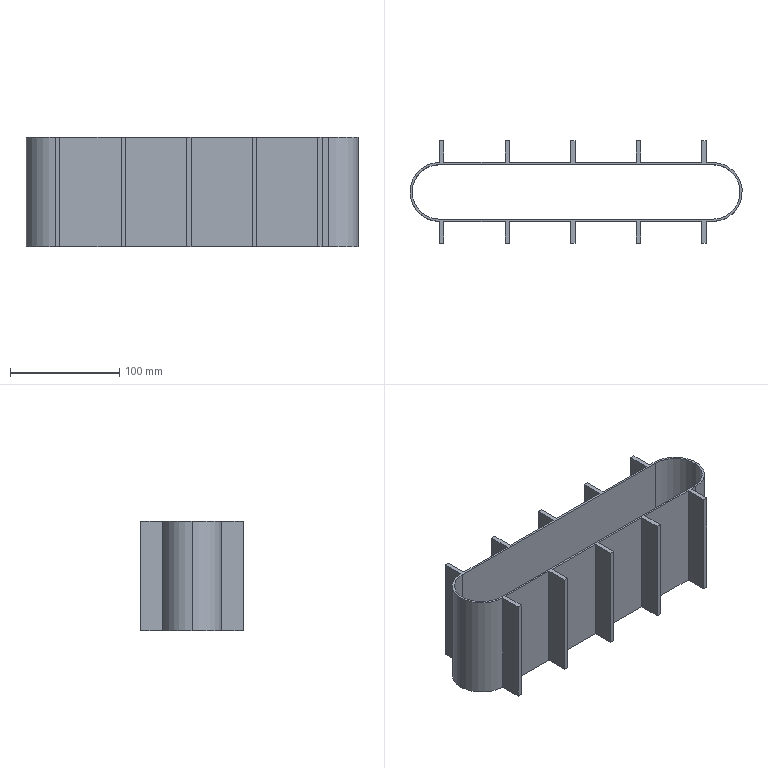Part | SolidWorks | features ICE 2, LPattern 2, Extrusion 1 | 1 solid | 50 faces | box 304 x 94 x 100 mm | volume 212673 mm3 | plane 44 | cylinder 6 | commonest cylinder face diameters 50 x3 54 x3
STEP:
#1=CARTESIAN_POINT('',(0.,25.,100.));
#2=VERTEX_POINT('',#1);
#3=CARTESIAN_POINT('',(-25.,0.,100.));
#4=VERTEX_POINT('',#3);
#5=CARTESIAN_POINT('',(0.,0.,100.));
#6=DIRECTION('',(0.,0.,1.));
#7=DIRECTION('',(1.,0.,0.));
#8=AXIS2_PLACEMENT_3D('',#5,#6,#7);
#9=CIRCLE('',#8,25.);
#10=EDGE_CURVE('',#2,#4,#9,.T.);
#11=ORIENTED_EDGE('',*,*,#10,.T.);
#12=CARTESIAN_POINT('',(-25.,0.,0.));
#13=VERTEX_POINT('',#12);
#14=CARTESIAN_POINT('',(-25.,0.,100.));
#15=DIRECTION('',(0.,0.,-1.));
#16=VECTOR('',#15,1000.);
#17=LINE('',#14,#16);
#18=EDGE_CURVE('',#4,#13,#17,.T.);
#19=ORIENTED_EDGE('',*,*,#18,.T.);
#20=CARTESIAN_POINT('',(0.,25.,0.));
#21=VERTEX_POINT('',#20);
#22=CARTESIAN_POINT('',(0.,0.,0.));
#23=DIRECTION('',(0.,0.,1.));
#24=DIRECTION('',(1.,0.,0.));
#25=AXIS2_PLACEMENT_3D('',#22,#23,#24);
#26=CIRCLE('',#25,25.);
#27=EDGE_CURVE('',#21,#13,#26,.T.);
#28=ORIENTED_EDGE('',*,*,#27,.F.);
#29=CARTESIAN_POINT('',(0.,25.,100.));
#30=DIRECTION('',(0.,0.,-1.));
#31=VECTOR('',#30,1000.);
#32=LINE('',#29,#31);
#33=EDGE_CURVE('',#2,#21,#32,.T.);
#34=ORIENTED_EDGE('',*,*,#33,.F.);
#35=EDGE_LOOP('',(#11,#19,#28,#34));
#36=FACE_OUTER_BOUND('',#35,.T.);
#37=CARTESIAN_POINT('',(0.,0.,100.));
#38=DIRECTION('',(0.,0.,-1.));
#39=DIRECTION('',(-1.,0.,0.));
#40=AXIS2_PLACEMENT_3D('',#37,#38,#39);
#41=CYLINDRICAL_SURFACE('',#40,25.);
#42=ADVANCED_FACE('',(#36),#41,.F.);
#43=CARTESIAN_POINT('',(-27.,0.,100.));
#44=VERTEX_POINT('',#43);
#45=CARTESIAN_POINT('',(0.,-27.,100.));
#46=VERTEX_POINT('',#45);
#47=CARTESIAN_POINT('',(0.,0.,100.));
#48=DIRECTION('',(0.,0.,1.));
#49=DIRECTION('',(1.,0.,0.));
#50=AXIS2_PLACEMENT_3D('',#47,#48,#49);
#51=CIRCLE('',#50,27.);
#52=EDGE_CURVE('',#44,#46,#51,.T.);
#53=ORIENTED_EDGE('',*,*,#52,.F.);
#54=CARTESIAN_POINT('',(-27.,0.,0.));
#55=VERTEX_POINT('',#54);
#56=CARTESIAN_POINT('',(-27.,0.,100.));
#57=DIRECTION('',(0.,0.,-1.));
#58=VECTOR('',#57,1000.);
#59=LINE('',#56,#58);
#60=EDGE_CURVE('',#44,#55,#59,.T.);
#61=ORIENTED_EDGE('',*,*,#60,.T.);
#62=CARTESIAN_POINT('',(0.,-27.,0.));
#63=VERTEX_POINT('',#62);
#64=CARTESIAN_POINT('',(0.,0.,0.));
#65=DIRECTION('',(0.,0.,1.));
#66=DIRECTION('',(1.,0.,0.));
#67=AXIS2_PLACEMENT_3D('',#64,#65,#66);
#68=CIRCLE('',#67,27.);
#69=EDGE_CURVE('',#55,#63,#68,.T.);
#70=ORIENTED_EDGE('',*,*,#69,.T.);
#71=CARTESIAN_POINT('',(0.,-27.,100.));
#72=DIRECTION('',(0.,0.,-1.));
#73=VECTOR('',#72,1000.);
#74=LINE('',#71,#73);
#75=EDGE_CURVE('',#46,#63,#74,.T.);
#76=ORIENTED_EDGE('',*,*,#75,.F.);
#77=EDGE_LOOP('',(#53,#61,#70,#76));
#78=FACE_OUTER_BOUND('',#77,.T.);
#79=CARTESIAN_POINT('',(0.,0.,100.));
#80=DIRECTION('',(0.,0.,-1.));
#81=DIRECTION('',(-1.,0.,0.));
#82=AXIS2_PLACEMENT_3D('',#79,#80,#81);
#83=CYLINDRICAL_SURFACE('',#82,27.);
#84=ADVANCED_FACE('',(#78),#83,.T.);
#85=CARTESIAN_POINT('',(184.,-27.,0.));
#86=VERTEX_POINT('',#85);
#87=CARTESIAN_POINT('',(240.,-27.,0.));
#88=VERTEX_POINT('',#87);
#89=CARTESIAN_POINT('',(0.,-27.,0.));
#90=DIRECTION('',(1.,0.,0.));
#91=VECTOR('',#90,1000.);
#92=LINE('',#89,#91);
#93=EDGE_CURVE('',#86,#88,#92,.T.);
#94=ORIENTED_EDGE('',*,*,#93,.T.);
#95=CARTESIAN_POINT('',(240.,-27.,100.));
#96=VERTEX_POINT('',#95);
#97=CARTESIAN_POINT('',(240.,-27.,-20.396));
#98=DIRECTION('',(0.,0.,1.));
#99=VECTOR('',#98,1000.);
#100=LINE('',#97,#99);
#101=EDGE_CURVE('',#88,#96,#100,.T.);
#102=ORIENTED_EDGE('',*,*,#101,.T.);
#103=CARTESIAN_POINT('',(184.,-27.,100.));
#104=VERTEX_POINT('',#103);
#105=CARTESIAN_POINT('',(0.,-27.,100.));
#106=DIRECTION('',(1.,0.,0.));
#107=VECTOR('',#106,1000.);
#108=LINE('',#105,#107);
#109=EDGE_CURVE('',#104,#96,#108,.T.);
#110=ORIENTED_EDGE('',*,*,#109,.F.);
#111=CARTESIAN_POINT('',(184.,-27.,-20.396));
#112=DIRECTION('',(0.,0.,1.));
#113=VECTOR('',#112,1000.);
#114=LINE('',#111,#113);
#115=EDGE_CURVE('',#86,#104,#114,.T.);
#116=ORIENTED_EDGE('',*,*,#115,.F.);
#117=EDGE_LOOP('',(#94,#102,#110,#116));
#118=FACE_OUTER_BOUND('',#117,.T.);
#119=CARTESIAN_POINT('',(0.,-27.,100.));
#120=DIRECTION('',(0.,1.,0.));
#121=DIRECTION('',(0.,0.,1.));
#122=AXIS2_PLACEMENT_3D('',#119,#120,#121);
#123=PLANE('',#122);
#124=ADVANCED_FACE('',(#118),#123,.F.);
#125=CARTESIAN_POINT('',(124.,-27.,0.));
#126=VERTEX_POINT('',#125);
#127=CARTESIAN_POINT('',(180.,-27.,0.));
#128=VERTEX_POINT('',#127);
#129=CARTESIAN_POINT('',(0.,-27.,0.));
#130=DIRECTION('',(1.,0.,0.));
#131=VECTOR('',#130,1000.);
#132=LINE('',#129,#131);
#133=EDGE_CURVE('',#126,#128,#132,.T.);
#134=ORIENTED_EDGE('',*,*,#133,.T.);
#135=CARTESIAN_POINT('',(180.,-27.,100.));
#136=VERTEX_POINT('',#135);
#137=CARTESIAN_POINT('',(180.,-27.,-20.396));
#138=DIRECTION('',(0.,0.,1.));
#139=VECTOR('',#138,1000.);
#140=LINE('',#137,#139);
#141=EDGE_CURVE('',#128,#136,#140,.T.);
#142=ORIENTED_EDGE('',*,*,#141,.T.);
#143=CARTESIAN_POINT('',(124.,-27.,100.));
#144=VERTEX_POINT('',#143);
#145=CARTESIAN_POINT('',(0.,-27.,100.));
#146=DIRECTION('',(1.,0.,0.));
#147=VECTOR('',#146,1000.);
#148=LINE('',#145,#147);
#149=EDGE_CURVE('',#144,#136,#148,.T.);
#150=ORIENTED_EDGE('',*,*,#149,.F.);
#151=CARTESIAN_POINT('',(124.,-27.,-20.396));
#152=DIRECTION('',(0.,0.,1.));
#153=VECTOR('',#152,1000.);
#154=LINE('',#151,#153);
#155=EDGE_CURVE('',#126,#144,#154,.T.);
#156=ORIENTED_EDGE('',*,*,#155,.F.);
#157=EDGE_LOOP('',(#134,#142,#150,#156));
#158=FACE_OUTER_BOUND('',#157,.T.);
#159=CARTESIAN_POINT('',(0.,-27.,100.));
#160=DIRECTION('',(0.,1.,0.));
#161=DIRECTION('',(0.,0.,1.));
#162=AXIS2_PLACEMENT_3D('',#159,#160,#161);
#163=PLANE('',#162);
#164=ADVANCED_FACE('',(#158),#163,.F.);
#165=CARTESIAN_POINT('',(64.,-27.,0.));
#166=VERTEX_POINT('',#165);
#167=CARTESIAN_POINT('',(120.,-27.,0.));
#168=VERTEX_POINT('',#167);
#169=CARTESIAN_POINT('',(0.,-27.,0.));
#170=DIRECTION('',(1.,0.,0.));
#171=VECTOR('',#170,1000.);
#172=LINE('',#169,#171);
#173=EDGE_CURVE('',#166,#168,#172,.T.);
#174=ORIENTED_EDGE('',*,*,#173,.T.);
#175=CARTESIAN_POINT('',(120.,-27.,100.));
#176=VERTEX_POINT('',#175);
#177=CARTESIAN_POINT('',(120.,-27.,-20.396));
#178=DIRECTION('',(0.,0.,1.));
#179=VECTOR('',#178,1000.);
#180=LINE('',#177,#179);
#181=EDGE_CURVE('',#168,#176,#180,.T.);
#182=ORIENTED_EDGE('',*,*,#181,.T.);
#183=CARTESIAN_POINT('',(64.,-27.,100.));
#184=VERTEX_POINT('',#183);
#185=CARTESIAN_POINT('',(0.,-27.,100.));
#186=DIRECTION('',(1.,0.,0.));
#187=VECTOR('',#186,1000.);
#188=LINE('',#185,#187);
#189=EDGE_CURVE('',#184,#176,#188,.T.);
#190=ORIENTED_EDGE('',*,*,#189,.F.);
#191=CARTESIAN_POINT('',(64.,-27.,-20.396));
#192=DIRECTION('',(0.,0.,1.));
#193=VECTOR('',#192,1000.);
#194=LINE('',#191,#193);
#195=EDGE_CURVE('',#166,#184,#194,.T.);
#196=ORIENTED_EDGE('',*,*,#195,.F.);
#197=EDGE_LOOP('',(#174,#182,#190,#196));
#198=FACE_OUTER_BOUND('',#197,.T.);
#199=CARTESIAN_POINT('',(0.,-27.,100.));
#200=DIRECTION('',(0.,1.,0.));
#201=DIRECTION('',(0.,0.,1.));
#202=AXIS2_PLACEMENT_3D('',#199,#200,#201);
#203=PLANE('',#202);
#204=ADVANCED_FACE('',(#198),#203,.F.);
#205=CARTESIAN_POINT('',(4.,-27.,0.));
#206=VERTEX_POINT('',#205);
#207=CARTESIAN_POINT('',(60.,-27.,0.));
#208=VERTEX_POINT('',#207);
#209=CARTESIAN_POINT('',(0.,-27.,0.));
#210=DIRECTION('',(1.,0.,0.));
#211=VECTOR('',#210,1000.);
#212=LINE('',#209,#211);
#213=EDGE_CURVE('',#206,#208,#212,.T.);
#214=ORIENTED_EDGE('',*,*,#213,.T.);
#215=CARTESIAN_POINT('',(60.,-27.,100.));
#216=VERTEX_POINT('',#215);
#217=CARTESIAN_POINT('',(60.,-27.,-20.396));
#218=DIRECTION('',(0.,0.,1.));
#219=VECTOR('',#218,1000.);
#220=LINE('',#217,#219);
#221=EDGE_CURVE('',#208,#216,#220,.T.);
#222=ORIENTED_EDGE('',*,*,#221,.T.);
#223=CARTESIAN_POINT('',(4.,-27.,100.));
#224=VERTEX_POINT('',#223);
#225=CARTESIAN_POINT('',(0.,-27.,100.));
#226=DIRECTION('',(1.,0.,0.));
#227=VECTOR('',#226,1000.);
#228=LINE('',#225,#227);
#229=EDGE_CURVE('',#224,#216,#228,.T.);
#230=ORIENTED_EDGE('',*,*,#229,.F.);
#231=CARTESIAN_POINT('',(4.,-27.,-20.396));
#232=DIRECTION('',(0.,0.,1.));
#233=VECTOR('',#232,1000.);
#234=LINE('',#231,#233);
#235=EDGE_CURVE('',#206,#224,#234,.T.);
#236=ORIENTED_EDGE('',*,*,#235,.F.);
#237=EDGE_LOOP('',(#214,#222,#230,#236));
#238=FACE_OUTER_BOUND('',#237,.T.);
#239=CARTESIAN_POINT('',(0.,-27.,100.));
#240=DIRECTION('',(0.,1.,0.));
#241=DIRECTION('',(0.,0.,1.));
#242=AXIS2_PLACEMENT_3D('',#239,#240,#241);
#243=PLANE('',#242);
#244=ADVANCED_FACE('',(#238),#243,.F.);
#245=CARTESIAN_POINT('',(240.,27.,100.));
#246=VERTEX_POINT('',#245);
#247=CARTESIAN_POINT('',(184.,27.,100.));
#248=VERTEX_POINT('',#247);
#249=CARTESIAN_POINT('',(0.,27.,100.));
#250=DIRECTION('',(-1.,0.,0.));
#251=VECTOR('',#250,1000.);
#252=LINE('',#249,#251);
#253=EDGE_CURVE('',#246,#248,#252,.T.);
#254=ORIENTED_EDGE('',*,*,#253,.F.);
#255=CARTESIAN_POINT('',(240.,27.,0.));
#256=VERTEX_POINT('',#255);
#257=CARTESIAN_POINT('',(240.,27.,-20.396));
#258=DIRECTION('',(0.,0.,1.));
#259=VECTOR('',#258,1000.);
#260=LINE('',#257,#259);
#261=EDGE_CURVE('',#256,#246,#260,.T.);
#262=ORIENTED_EDGE('',*,*,#261,.F.);
#263=CARTESIAN_POINT('',(184.,27.,0.));
#264=VERTEX_POINT('',#263);
#265=CARTESIAN_POINT('',(0.,27.,0.));
#266=DIRECTION('',(-1.,0.,0.));
#267=VECTOR('',#266,1000.);
#268=LINE('',#265,#267);
#269=EDGE_CURVE('',#256,#264,#268,.T.);
#270=ORIENTED_EDGE('',*,*,#269,.T.);
#271=CARTESIAN_POINT('',(184.,27.,-20.396));
#272=DIRECTION('',(0.,0.,1.));
#273=VECTOR('',#272,1000.);
#274=LINE('',#271,#273);
#275=EDGE_CURVE('',#264,#248,#274,.T.);
#276=ORIENTED_EDGE('',*,*,#275,.T.);
#277=EDGE_LOOP('',(#254,#262,#270,#276));
#278=FACE_OUTER_BOUND('',#277,.T.);
#279=CARTESIAN_POINT('',(0.,27.,100.));
#280=DIRECTION('',(0.,-1.,0.));
#281=DIRECTION('',(0.,0.,-1.));
#282=AXIS2_PLACEMENT_3D('',#279,#280,#281);
#283=PLANE('',#282);
#284=ADVANCED_FACE('',(#278),#283,.F.);
#285=CARTESIAN_POINT('',(180.,27.,100.));
#286=VERTEX_POINT('',#285);
#287=CARTESIAN_POINT('',(124.,27.,100.));
#288=VERTEX_POINT('',#287);
#289=CARTESIAN_POINT('',(0.,27.,100.));
#290=DIRECTION('',(-1.,0.,0.));
#291=VECTOR('',#290,1000.);
#292=LINE('',#289,#291);
#293=EDGE_CURVE('',#286,#288,#292,.T.);
#294=ORIENTED_EDGE('',*,*,#293,.F.);
#295=CARTESIAN_POINT('',(180.,27.,0.));
#296=VERTEX_POINT('',#295);
#297=CARTESIAN_POINT('',(180.,27.,-20.396));
#298=DIRECTION('',(0.,0.,1.));
#299=VECTOR('',#298,1000.);
#300=LINE('',#297,#299);
#301=EDGE_CURVE('',#296,#286,#300,.T.);
#302=ORIENTED_EDGE('',*,*,#301,.F.);
#303=CARTESIAN_POINT('',(124.,27.,0.));
#304=VERTEX_POINT('',#303);
#305=CARTESIAN_POINT('',(0.,27.,0.));
#306=DIRECTION('',(-1.,0.,0.));
#307=VECTOR('',#306,1000.);
#308=LINE('',#305,#307);
#309=EDGE_CURVE('',#296,#304,#308,.T.);
#310=ORIENTED_EDGE('',*,*,#309,.T.);
#311=CARTESIAN_POINT('',(124.,27.,-20.396));
#312=DIRECTION('',(0.,0.,1.));
#313=VECTOR('',#312,1000.);
#314=LINE('',#311,#313);
#315=EDGE_CURVE('',#304,#288,#314,.T.);
#316=ORIENTED_EDGE('',*,*,#315,.T.);
#317=EDGE_LOOP('',(#294,#302,#310,#316));
#318=FACE_OUTER_BOUND('',#317,.T.);
#319=CARTESIAN_POINT('',(0.,27.,100.));
#320=DIRECTION('',(0.,-1.,0.));
#321=DIRECTION('',(0.,0.,-1.));
#322=AXIS2_PLACEMENT_3D('',#319,#320,#321);
#323=PLANE('',#322);
#324=ADVANCED_FACE('',(#318),#323,.F.);
#325=CARTESIAN_POINT('',(120.,27.,100.));
#326=VERTEX_POINT('',#325);
#327=CARTESIAN_POINT('',(64.,27.,100.));
#328=VERTEX_POINT('',#327);
#329=CARTESIAN_POINT('',(0.,27.,100.));
#330=DIRECTION('',(-1.,0.,0.));
#331=VECTOR('',#330,1000.);
#332=LINE('',#329,#331);
#333=EDGE_CURVE('',#326,#328,#332,.T.);
#334=ORIENTED_EDGE('',*,*,#333,.F.);
#335=CARTESIAN_POINT('',(120.,27.,0.));
#336=VERTEX_POINT('',#335);
#337=CARTESIAN_POINT('',(120.,27.,-20.396));
#338=DIRECTION('',(0.,0.,1.));
#339=VECTOR('',#338,1000.);
#340=LINE('',#337,#339);
#341=EDGE_CURVE('',#336,#326,#340,.T.);
#342=ORIENTED_EDGE('',*,*,#341,.F.);
#343=CARTESIAN_POINT('',(64.,27.,0.));
#344=VERTEX_POINT('',#343);
#345=CARTESIAN_POINT('',(0.,27.,0.));
#346=DIRECTION('',(-1.,0.,0.));
#347=VECTOR('',#346,1000.);
#348=LINE('',#345,#347);
#349=EDGE_CURVE('',#336,#344,#348,.T.);
#350=ORIENTED_EDGE('',*,*,#349,.T.);
#351=CARTESIAN_POINT('',(64.,27.,-20.396));
#352=DIRECTION('',(0.,0.,1.));
#353=VECTOR('',#352,1000.);
#354=LINE('',#351,#353);
#355=EDGE_CURVE('',#344,#328,#354,.T.);
#356=ORIENTED_EDGE('',*,*,#355,.T.);
#357=EDGE_LOOP('',(#334,#342,#350,#356));
#358=FACE_OUTER_BOUND('',#357,.T.);
#359=CARTESIAN_POINT('',(0.,27.,100.));
#360=DIRECTION('',(0.,-1.,0.));
#361=DIRECTION('',(0.,0.,-1.));
#362=AXIS2_PLACEMENT_3D('',#359,#360,#361);
#363=PLANE('',#362);
#364=ADVANCED_FACE('',(#358),#363,.F.);
#365=CARTESIAN_POINT('',(60.,27.,100.));
#366=VERTEX_POINT('',#365);
#367=CARTESIAN_POINT('',(4.,27.,100.));
#368=VERTEX_POINT('',#367);
#369=CARTESIAN_POINT('',(0.,27.,100.));
#370=DIRECTION('',(-1.,0.,0.));
#371=VECTOR('',#370,1000.);
#372=LINE('',#369,#371);
#373=EDGE_CURVE('',#366,#368,#372,.T.);
#374=ORIENTED_EDGE('',*,*,#373,.F.);
#375=CARTESIAN_POINT('',(60.,27.,0.));
#376=VERTEX_POINT('',#375);
#377=CARTESIAN_POINT('',(60.,27.,-20.396));
#378=DIRECTION('',(0.,0.,1.));
#379=VECTOR('',#378,1000.);
#380=LINE('',#377,#379);
#381=EDGE_CURVE('',#376,#366,#380,.T.);
#382=ORIENTED_EDGE('',*,*,#381,.F.);
#383=CARTESIAN_POINT('',(4.,27.,0.));
#384=VERTEX_POINT('',#383);
#385=CARTESIAN_POINT('',(0.,27.,0.));
#386=DIRECTION('',(-1.,0.,0.));
#387=VECTOR('',#386,1000.);
#388=LINE('',#385,#387);
#389=EDGE_CURVE('',#376,#384,#388,.T.);
#390=ORIENTED_EDGE('',*,*,#389,.T.);
#391=CARTESIAN_POINT('',(4.,27.,-20.396));
#392=DIRECTION('',(0.,0.,1.));
#393=VECTOR('',#392,1000.);
#394=LINE('',#391,#393);
#395=EDGE_CURVE('',#384,#368,#394,.T.);
#396=ORIENTED_EDGE('',*,*,#395,.T.);
#397=EDGE_LOOP('',(#374,#382,#390,#396));
#398=FACE_OUTER_BOUND('',#397,.T.);
#399=CARTESIAN_POINT('',(0.,27.,100.));
#400=DIRECTION('',(0.,-1.,0.));
#401=DIRECTION('',(0.,0.,-1.));
#402=AXIS2_PLACEMENT_3D('',#399,#400,#401);
#403=PLANE('',#402);
#404=ADVANCED_FACE('',(#398),#403,.F.);
#405=CARTESIAN_POINT('',(0.,27.,100.));
#406=VERTEX_POINT('',#405);
#407=CARTESIAN_POINT('',(0.,0.,100.));
#408=DIRECTION('',(0.,0.,1.));
#409=DIRECTION('',(1.,0.,0.));
#410=AXIS2_PLACEMENT_3D('',#407,#408,#409);
#411=CIRCLE('',#410,27.);
#412=EDGE_CURVE('',#406,#44,#411,.T.);
#413=ORIENTED_EDGE('',*,*,#412,.T.);
#414=ORIENTED_EDGE('',*,*,#52,.T.);
#415=CARTESIAN_POINT('',(0.,-47.,100.));
#416=VERTEX_POINT('',#415);
#417=CARTESIAN_POINT('',(0.,-27.,100.));
#418=DIRECTION('',(0.,-1.,0.));
#419=VECTOR('',#418,1000.);
#420=LINE('',#417,#419);
#421=EDGE_CURVE('',#46,#416,#420,.T.);
#422=ORIENTED_EDGE('',*,*,#421,.T.);
#423=CARTESIAN_POINT('',(4.,-47.,100.));
#424=VERTEX_POINT('',#423);
#425=CARTESIAN_POINT('',(0.,-47.,100.));
#426=DIRECTION('',(1.,0.,0.));
#427=VECTOR('',#426,1000.);
#428=LINE('',#425,#427);
#429=EDGE_CURVE('',#416,#424,#428,.T.);
#430=ORIENTED_EDGE('',*,*,#429,.T.);
#431=CARTESIAN_POINT('',(4.,-27.,100.));
#432=DIRECTION('',(0.,1.,0.));
#433=VECTOR('',#432,1000.);
#434=LINE('',#431,#433);
#435=EDGE_CURVE('',#424,#224,#434,.T.);
#436=ORIENTED_EDGE('',*,*,#435,.T.);
#437=ORIENTED_EDGE('',*,*,#229,.T.);
#438=CARTESIAN_POINT('',(60.,-47.,100.));
#439=VERTEX_POINT('',#438);
#440=CARTESIAN_POINT('',(60.,-27.,100.));
#441=DIRECTION('',(0.,-1.,0.));
#442=VECTOR('',#441,1000.);
#443=LINE('',#440,#442);
#444=EDGE_CURVE('',#216,#439,#443,.T.);
#445=ORIENTED_EDGE('',*,*,#444,.T.);
#446=CARTESIAN_POINT('',(64.,-47.,100.));
#447=VERTEX_POINT('',#446);
#448=CARTESIAN_POINT('',(60.,-47.,100.));
#449=DIRECTION('',(1.,0.,0.));
#450=VECTOR('',#449,1000.);
#451=LINE('',#448,#450);
#452=EDGE_CURVE('',#439,#447,#451,.T.);
#453=ORIENTED_EDGE('',*,*,#452,.T.);
#454=CARTESIAN_POINT('',(64.,-27.,100.));
#455=DIRECTION('',(0.,1.,0.));
#456=VECTOR('',#455,1000.);
#457=LINE('',#454,#456);
#458=EDGE_CURVE('',#447,#184,#457,.T.);
#459=ORIENTED_EDGE('',*,*,#458,.T.);
#460=ORIENTED_EDGE('',*,*,#189,.T.);
#461=CARTESIAN_POINT('',(120.,-47.,100.));
#462=VERTEX_POINT('',#461);
#463=CARTESIAN_POINT('',(120.,-27.,100.));
#464=DIRECTION('',(0.,-1.,0.));
#465=VECTOR('',#464,1000.);
#466=LINE('',#463,#465);
#467=EDGE_CURVE('',#176,#462,#466,.T.);
#468=ORIENTED_EDGE('',*,*,#467,.T.);
#469=CARTESIAN_POINT('',(124.,-47.,100.));
#470=VERTEX_POINT('',#469);
#471=CARTESIAN_POINT('',(120.,-47.,100.));
#472=DIRECTION('',(1.,0.,0.));
#473=VECTOR('',#472,1000.);
#474=LINE('',#471,#473);
#475=EDGE_CURVE('',#462,#470,#474,.T.);
#476=ORIENTED_EDGE('',*,*,#475,.T.);
#477=CARTESIAN_POINT('',(124.,-27.,100.));
#478=DIRECTION('',(0.,1.,0.));
#479=VECTOR('',#478,1000.);
#480=LINE('',#477,#479);
#481=EDGE_CURVE('',#470,#144,#480,.T.);
#482=ORIENTED_EDGE('',*,*,#481,.T.);
#483=ORIENTED_EDGE('',*,*,#149,.T.);
#484=CARTESIAN_POINT('',(180.,-47.,100.));
#485=VERTEX_POINT('',#484);
#486=CARTESIAN_POINT('',(180.,-27.,100.));
#487=DIRECTION('',(0.,-1.,0.));
#488=VECTOR('',#487,1000.);
#489=LINE('',#486,#488);
#490=EDGE_CURVE('',#136,#485,#489,.T.);
#491=ORIENTED_EDGE('',*,*,#490,.T.);
#492=CARTESIAN_POINT('',(184.,-47.,100.));
#493=VERTEX_POINT('',#492);
#494=CARTESIAN_POINT('',(180.,-47.,100.));
#495=DIRECTION('',(1.,0.,0.));
#496=VECTOR('',#495,1000.);
#497=LINE('',#494,#496);
#498=EDGE_CURVE('',#485,#493,#497,.T.);
#499=ORIENTED_EDGE('',*,*,#498,.T.);
#500=CARTESIAN_POINT('',(184.,-27.,100.));
#501=DIRECTION('',(0.,1.,0.));
#502=VECTOR('',#501,1000.);
#503=LINE('',#500,#502);
#504=EDGE_CURVE('',#493,#104,#503,.T.);
#505=ORIENTED_EDGE('',*,*,#504,.T.);
#506=ORIENTED_EDGE('',*,*,#109,.T.);
#507=CARTESIAN_POINT('',(240.,-47.,100.));
#508=VERTEX_POINT('',#507);
#509=CARTESIAN_POINT('',(240.,-27.,100.));
#510=DIRECTION('',(0.,-1.,0.));
#511=VECTOR('',#510,1000.);
#512=LINE('',#509,#511);
#513=EDGE_CURVE('',#96,#508,#512,.T.);
#514=ORIENTED_EDGE('',*,*,#513,.T.);
#515=CARTESIAN_POINT('',(244.,-47.,100.));
#516=VERTEX_POINT('',#515);
#517=CARTESIAN_POINT('',(240.,-47.,100.));
#518=DIRECTION('',(1.,0.,0.));
#519=VECTOR('',#518,1000.);
#520=LINE('',#517,#519);
#521=EDGE_CURVE('',#508,#516,#520,.T.);
#522=ORIENTED_EDGE('',*,*,#521,.T.);
#523=CARTESIAN_POINT('',(244.,-27.,100.));
#524=VERTEX_POINT('',#523);
#525=CARTESIAN_POINT('',(244.,-27.,100.));
#526=DIRECTION('',(0.,1.,0.));
#527=VECTOR('',#526,1000.);
#528=LINE('',#525,#527);
#529=EDGE_CURVE('',#516,#524,#528,.T.);
#530=ORIENTED_EDGE('',*,*,#529,.T.);
#531=CARTESIAN_POINT('',(250.,-27.,100.));
#532=VERTEX_POINT('',#531);
#533=CARTESIAN_POINT('',(0.,-27.,100.));
#534=DIRECTION('',(1.,0.,0.));
#535=VECTOR('',#534,1000.);
#536=LINE('',#533,#535);
#537=EDGE_CURVE('',#524,#532,#536,.T.);
#538=ORIENTED_EDGE('',*,*,#537,.T.);
#539=CARTESIAN_POINT('',(250.,27.,100.));
#540=VERTEX_POINT('',#539);
#541=CARTESIAN_POINT('',(250.,0.,100.));
#542=DIRECTION('',(0.,0.,1.));
#543=DIRECTION('',(1.,0.,0.));
#544=AXIS2_PLACEMENT_3D('',#541,#542,#543);
#545=CIRCLE('',#544,27.);
#546=EDGE_CURVE('',#532,#540,#545,.T.);
#547=ORIENTED_EDGE('',*,*,#546,.T.);
#548=CARTESIAN_POINT('',(244.,27.,100.));
#549=VERTEX_POINT('',#548);
#550=CARTESIAN_POINT('',(0.,27.,100.));
#551=DIRECTION('',(-1.,0.,0.));
#552=VECTOR('',#551,1000.);
#553=LINE('',#550,#552);
#554=EDGE_CURVE('',#540,#549,#553,.T.);
#555=ORIENTED_EDGE('',*,*,#554,.T.);
#556=CARTESIAN_POINT('',(244.,47.,100.));
#557=VERTEX_POINT('',#556);
#558=CARTESIAN_POINT('',(244.,27.,100.));
#559=DIRECTION('',(0.,1.,0.));
#560=VECTOR('',#559,1000.);
#561=LINE('',#558,#560);
#562=EDGE_CURVE('',#549,#557,#561,.T.);
#563=ORIENTED_EDGE('',*,*,#562,.T.);
#564=CARTESIAN_POINT('',(240.,47.,100.));
#565=VERTEX_POINT('',#564);
#566=CARTESIAN_POINT('',(240.,47.,100.));
#567=DIRECTION('',(-1.,0.,0.));
#568=VECTOR('',#567,1000.);
#569=LINE('',#566,#568);
#570=EDGE_CURVE('',#557,#565,#569,.T.);
#571=ORIENTED_EDGE('',*,*,#570,.T.);
#572=CARTESIAN_POINT('',(240.,27.,100.));
#573=DIRECTION('',(0.,-1.,0.));
#574=VECTOR('',#573,1000.);
#575=LINE('',#572,#574);
#576=EDGE_CURVE('',#565,#246,#575,.T.);
#577=ORIENTED_EDGE('',*,*,#576,.T.);
#578=ORIENTED_EDGE('',*,*,#253,.T.);
#579=CARTESIAN_POINT('',(184.,47.,100.));
#580=VERTEX_POINT('',#579);
#581=CARTESIAN_POINT('',(184.,27.,100.));
#582=DIRECTION('',(0.,1.,0.));
#583=VECTOR('',#582,1000.);
#584=LINE('',#581,#583);
#585=EDGE_CURVE('',#248,#580,#584,.T.);
#586=ORIENTED_EDGE('',*,*,#585,.T.);
#587=CARTESIAN_POINT('',(180.,47.,100.));
#588=VERTEX_POINT('',#587);
#589=CARTESIAN_POINT('',(180.,47.,100.));
#590=DIRECTION('',(-1.,0.,0.));
#591=VECTOR('',#590,1000.);
#592=LINE('',#589,#591);
#593=EDGE_CURVE('',#580,#588,#592,.T.);
#594=ORIENTED_EDGE('',*,*,#593,.T.);
#595=CARTESIAN_POINT('',(180.,27.,100.));
#596=DIRECTION('',(0.,-1.,0.));
#597=VECTOR('',#596,1000.);
#598=LINE('',#595,#597);
#599=EDGE_CURVE('',#588,#286,#598,.T.);
#600=ORIENTED_EDGE('',*,*,#599,.T.);
#601=ORIENTED_EDGE('',*,*,#293,.T.);
#602=CARTESIAN_POINT('',(124.,47.,100.));
#603=VERTEX_POINT('',#602);
#604=CARTESIAN_POINT('',(124.,27.,100.));
#605=DIRECTION('',(0.,1.,0.));
#606=VECTOR('',#605,1000.);
#607=LINE('',#604,#606);
#608=EDGE_CURVE('',#288,#603,#607,.T.);
#609=ORIENTED_EDGE('',*,*,#608,.T.);
#610=CARTESIAN_POINT('',(120.,47.,100.));
#611=VERTEX_POINT('',#610);
#612=CARTESIAN_POINT('',(120.,47.,100.));
#613=DIRECTION('',(-1.,0.,0.));
#614=VECTOR('',#613,1000.);
#615=LINE('',#612,#614);
#616=EDGE_CURVE('',#603,#611,#615,.T.);
#617=ORIENTED_EDGE('',*,*,#616,.T.);
#618=CARTESIAN_POINT('',(120.,27.,100.));
#619=DIRECTION('',(0.,-1.,0.));
#620=VECTOR('',#619,1000.);
#621=LINE('',#618,#620);
#622=EDGE_CURVE('',#611,#326,#621,.T.);
#623=ORIENTED_EDGE('',*,*,#622,.T.);
#624=ORIENTED_EDGE('',*,*,#333,.T.);
#625=CARTESIAN_POINT('',(64.,47.,100.));
#626=VERTEX_POINT('',#625);
#627=CARTESIAN_POINT('',(64.,27.,100.));
#628=DIRECTION('',(0.,1.,0.));
#629=VECTOR('',#628,1000.);
#630=LINE('',#627,#629);
#631=EDGE_CURVE('',#328,#626,#630,.T.);
#632=ORIENTED_EDGE('',*,*,#631,.T.);
#633=CARTESIAN_POINT('',(60.,47.,100.));
#634=VERTEX_POINT('',#633);
#635=CARTESIAN_POINT('',(60.,47.,100.));
#636=DIRECTION('',(-1.,0.,0.));
#637=VECTOR('',#636,1000.);
#638=LINE('',#635,#637);
#639=EDGE_CURVE('',#626,#634,#638,.T.);
#640=ORIENTED_EDGE('',*,*,#639,.T.);
#641=CARTESIAN_POINT('',(60.,27.,100.));
#642=DIRECTION('',(0.,-1.,0.));
#643=VECTOR('',#642,1000.);
#644=LINE('',#641,#643);
#645=EDGE_CURVE('',#634,#366,#644,.T.);
#646=ORIENTED_EDGE('',*,*,#645,.T.);
#647=ORIENTED_EDGE('',*,*,#373,.T.);
#648=CARTESIAN_POINT('',(4.,47.,100.));
#649=VERTEX_POINT('',#648);
#650=CARTESIAN_POINT('',(4.,27.,100.));
#651=DIRECTION('',(0.,1.,0.));
#652=VECTOR('',#651,1000.);
#653=LINE('',#650,#652);
#654=EDGE_CURVE('',#368,#649,#653,.T.);
#655=ORIENTED_EDGE('',*,*,#654,.T.);
#656=CARTESIAN_POINT('',(0.,47.,100.));
#657=VERTEX_POINT('',#656);
#658=CARTESIAN_POINT('',(0.,47.,100.));
#659=DIRECTION('',(-1.,0.,0.));
#660=VECTOR('',#659,1000.);
#661=LINE('',#658,#660);
#662=EDGE_CURVE('',#649,#657,#661,.T.);
#663=ORIENTED_EDGE('',*,*,#662,.T.);
#664=CARTESIAN_POINT('',(0.,27.,100.));
#665=DIRECTION('',(0.,-1.,0.));
#666=VECTOR('',#665,1000.);
#667=LINE('',#664,#666);
#668=EDGE_CURVE('',#657,#406,#667,.T.);
#669=ORIENTED_EDGE('',*,*,#668,.T.);
#670=EDGE_LOOP('',(#413,#414,#422,#430,#436,#437,#445,#453,#459,#460,#468,#476,#482,#483,#491,#499,#505,#506,#514,#522,#530,#538,#547,#555,#563,#571,#577,#578,#586,#594,#600,#601,#609,#617,#623,#624,#632,#640,#646,#647,#655,#663,#669));
#671=FACE_OUTER_BOUND('',#670,.T.);
#672=CARTESIAN_POINT('',(0.,-25.,100.));
#673=VERTEX_POINT('',#672);
#674=CARTESIAN_POINT('',(250.,-25.,100.));
#675=VERTEX_POINT('',#674);
#676=CARTESIAN_POINT('',(0.,-25.,100.));
#677=DIRECTION('',(1.,0.,0.));
#678=VECTOR('',#677,1000.);
#679=LINE('',#676,#678);
#680=EDGE_CURVE('',#673,#675,#679,.T.);
#681=ORIENTED_EDGE('',*,*,#680,.F.);
#682=CARTESIAN_POINT('',(0.,0.,100.));
#683=DIRECTION('',(0.,0.,1.));
#684=DIRECTION('',(1.,0.,0.));
#685=AXIS2_PLACEMENT_3D('',#682,#683,#684);
#686=CIRCLE('',#685,25.);
#687=EDGE_CURVE('',#4,#673,#686,.T.);
#688=ORIENTED_EDGE('',*,*,#687,.F.);
#689=ORIENTED_EDGE('',*,*,#10,.F.);
#690=CARTESIAN_POINT('',(250.,25.,100.));
#691=VERTEX_POINT('',#690);
#692=CARTESIAN_POINT('',(0.,25.,100.));
#693=DIRECTION('',(-1.,0.,0.));
#694=VECTOR('',#693,1000.);
#695=LINE('',#692,#694);
#696=EDGE_CURVE('',#691,#2,#695,.T.);
#697=ORIENTED_EDGE('',*,*,#696,.F.);
#698=CARTESIAN_POINT('',(250.,0.,100.));
#699=DIRECTION('',(0.,0.,1.));
#700=DIRECTION('',(1.,0.,0.));
#701=AXIS2_PLACEMENT_3D('',#698,#699,#700);
#702=CIRCLE('',#701,25.);
#703=EDGE_CURVE('',#675,#691,#702,.T.);
#704=ORIENTED_EDGE('',*,*,#703,.F.);
#705=EDGE_LOOP('',(#681,#688,#689,#697,#704));
#706=FACE_BOUND('',#705,.T.);
#707=CARTESIAN_POINT('',(0.,0.,100.));
#708=DIRECTION('',(0.,0.,1.));
#709=DIRECTION('',(1.,0.,0.));
#710=AXIS2_PLACEMENT_3D('',#707,#708,#709);
#711=PLANE('',#710);
#712=ADVANCED_FACE('',(#671,#706),#711,.T.);
#713=CARTESIAN_POINT('',(0.,27.,0.));
#714=VERTEX_POINT('',#713);
#715=CARTESIAN_POINT('',(0.,0.,0.));
#716=DIRECTION('',(0.,0.,1.));
#717=DIRECTION('',(1.,0.,0.));
#718=AXIS2_PLACEMENT_3D('',#715,#716,#717);
#719=CIRCLE('',#718,27.);
#720=EDGE_CURVE('',#714,#55,#719,.T.);
#721=ORIENTED_EDGE('',*,*,#720,.F.);
#722=CARTESIAN_POINT('',(0.,47.,0.));
#723=VERTEX_POINT('',#722);
#724=CARTESIAN_POINT('',(0.,27.,0.));
#725=DIRECTION('',(0.,1.,0.));
#726=VECTOR('',#725,1000.);
#727=LINE('',#724,#726);
#728=EDGE_CURVE('',#714,#723,#727,.T.);
#729=ORIENTED_EDGE('',*,*,#728,.T.);
#730=CARTESIAN_POINT('',(4.,47.,0.));
#731=VERTEX_POINT('',#730);
#732=CARTESIAN_POINT('',(0.,47.,0.));
#733=DIRECTION('',(1.,0.,0.));
#734=VECTOR('',#733,1000.);
#735=LINE('',#732,#734);
#736=EDGE_CURVE('',#723,#731,#735,.T.);
#737=ORIENTED_EDGE('',*,*,#736,.T.);
#738=CARTESIAN_POINT('',(4.,27.,0.));
#739=DIRECTION('',(0.,-1.,0.));
#740=VECTOR('',#739,1000.);
#741=LINE('',#738,#740);
#742=EDGE_CURVE('',#731,#384,#741,.T.);
#743=ORIENTED_EDGE('',*,*,#742,.T.);
#744=ORIENTED_EDGE('',*,*,#389,.F.);
#745=CARTESIAN_POINT('',(60.,47.,0.));
#746=VERTEX_POINT('',#745);
#747=CARTESIAN_POINT('',(60.,27.,0.));
#748=DIRECTION('',(0.,1.,0.));
#749=VECTOR('',#748,1000.);
#750=LINE('',#747,#749);
#751=EDGE_CURVE('',#376,#746,#750,.T.);
#752=ORIENTED_EDGE('',*,*,#751,.T.);
#753=CARTESIAN_POINT('',(64.,47.,0.));
#754=VERTEX_POINT('',#753);
#755=CARTESIAN_POINT('',(60.,47.,0.));
#756=DIRECTION('',(1.,0.,0.));
#757=VECTOR('',#756,1000.);
#758=LINE('',#755,#757);
#759=EDGE_CURVE('',#746,#754,#758,.T.);
#760=ORIENTED_EDGE('',*,*,#759,.T.);
#761=CARTESIAN_POINT('',(64.,27.,0.));
#762=DIRECTION('',(0.,-1.,0.));
#763=VECTOR('',#762,1000.);
#764=LINE('',#761,#763);
#765=EDGE_CURVE('',#754,#344,#764,.T.);
#766=ORIENTED_EDGE('',*,*,#765,.T.);
#767=ORIENTED_EDGE('',*,*,#349,.F.);
#768=CARTESIAN_POINT('',(120.,47.,0.));
#769=VERTEX_POINT('',#768);
#770=CARTESIAN_POINT('',(120.,27.,0.));
#771=DIRECTION('',(0.,1.,0.));
#772=VECTOR('',#771,1000.);
#773=LINE('',#770,#772);
#774=EDGE_CURVE('',#336,#769,#773,.T.);
#775=ORIENTED_EDGE('',*,*,#774,.T.);
#776=CARTESIAN_POINT('',(124.,47.,0.));
#777=VERTEX_POINT('',#776);
#778=CARTESIAN_POINT('',(120.,47.,0.));
#779=DIRECTION('',(1.,0.,0.));
#780=VECTOR('',#779,1000.);
#781=LINE('',#778,#780);
#782=EDGE_CURVE('',#769,#777,#781,.T.);
#783=ORIENTED_EDGE('',*,*,#782,.T.);
#784=CARTESIAN_POINT('',(124.,27.,0.));
#785=DIRECTION('',(0.,-1.,0.));
#786=VECTOR('',#785,1000.);
#787=LINE('',#784,#786);
#788=EDGE_CURVE('',#777,#304,#787,.T.);
#789=ORIENTED_EDGE('',*,*,#788,.T.);
#790=ORIENTED_EDGE('',*,*,#309,.F.);
#791=CARTESIAN_POINT('',(180.,47.,0.));
#792=VERTEX_POINT('',#791);
#793=CARTESIAN_POINT('',(180.,27.,0.));
#794=DIRECTION('',(0.,1.,0.));
#795=VECTOR('',#794,1000.);
#796=LINE('',#793,#795);
#797=EDGE_CURVE('',#296,#792,#796,.T.);
#798=ORIENTED_EDGE('',*,*,#797,.T.);
#799=CARTESIAN_POINT('',(184.,47.,0.));
#800=VERTEX_POINT('',#799);
#801=CARTESIAN_POINT('',(180.,47.,0.));
#802=DIRECTION('',(1.,0.,0.));
#803=VECTOR('',#802,1000.);
#804=LINE('',#801,#803);
#805=EDGE_CURVE('',#792,#800,#804,.T.);
#806=ORIENTED_EDGE('',*,*,#805,.T.);
#807=CARTESIAN_POINT('',(184.,27.,0.));
#808=DIRECTION('',(0.,-1.,0.));
#809=VECTOR('',#808,1000.);
#810=LINE('',#807,#809);
#811=EDGE_CURVE('',#800,#264,#810,.T.);
#812=ORIENTED_EDGE('',*,*,#811,.T.);
#813=ORIENTED_EDGE('',*,*,#269,.F.);
#814=CARTESIAN_POINT('',(240.,47.,0.));
#815=VERTEX_POINT('',#814);
#816=CARTESIAN_POINT('',(240.,27.,0.));
#817=DIRECTION('',(0.,1.,0.));
#818=VECTOR('',#817,1000.);
#819=LINE('',#816,#818);
#820=EDGE_CURVE('',#256,#815,#819,.T.);
#821=ORIENTED_EDGE('',*,*,#820,.T.);
#822=CARTESIAN_POINT('',(244.,47.,0.));
#823=VERTEX_POINT('',#822);
#824=CARTESIAN_POINT('',(240.,47.,0.));
#825=DIRECTION('',(1.,0.,0.));
#826=VECTOR('',#825,1000.);
#827=LINE('',#824,#826);
#828=EDGE_CURVE('',#815,#823,#827,.T.);
#829=ORIENTED_EDGE('',*,*,#828,.T.);
#830=CARTESIAN_POINT('',(244.,27.,0.));
#831=VERTEX_POINT('',#830);
#832=CARTESIAN_POINT('',(244.,27.,0.));
#833=DIRECTION('',(0.,-1.,0.));
#834=VECTOR('',#833,1000.);
#835=LINE('',#832,#834);
#836=EDGE_CURVE('',#823,#831,#835,.T.);
#837=ORIENTED_EDGE('',*,*,#836,.T.);
#838=CARTESIAN_POINT('',(250.,27.,0.));
#839=VERTEX_POINT('',#838);
#840=CARTESIAN_POINT('',(0.,27.,0.));
#841=DIRECTION('',(-1.,0.,0.));
#842=VECTOR('',#841,1000.);
#843=LINE('',#840,#842);
#844=EDGE_CURVE('',#839,#831,#843,.T.);
#845=ORIENTED_EDGE('',*,*,#844,.F.);
#846=CARTESIAN_POINT('',(250.,-27.,0.));
#847=VERTEX_POINT('',#846);
#848=CARTESIAN_POINT('',(250.,0.,0.));
#849=DIRECTION('',(0.,0.,1.));
#850=DIRECTION('',(1.,0.,0.));
#851=AXIS2_PLACEMENT_3D('',#848,#849,#850);
#852=CIRCLE('',#851,27.);
#853=EDGE_CURVE('',#847,#839,#852,.T.);
#854=ORIENTED_EDGE('',*,*,#853,.F.);
#855=CARTESIAN_POINT('',(244.,-27.,0.));
#856=VERTEX_POINT('',#855);
#857=CARTESIAN_POINT('',(0.,-27.,0.));
#858=DIRECTION('',(1.,0.,0.));
#859=VECTOR('',#858,1000.);
#860=LINE('',#857,#859);
#861=EDGE_CURVE('',#856,#847,#860,.T.);
#862=ORIENTED_EDGE('',*,*,#861,.F.);
#863=CARTESIAN_POINT('',(244.,-47.,0.));
#864=VERTEX_POINT('',#863);
#865=CARTESIAN_POINT('',(244.,-27.,0.));
#866=DIRECTION('',(0.,-1.,0.));
#867=VECTOR('',#866,1000.);
#868=LINE('',#865,#867);
#869=EDGE_CURVE('',#856,#864,#868,.T.);
#870=ORIENTED_EDGE('',*,*,#869,.T.);
#871=CARTESIAN_POINT('',(240.,-47.,0.));
#872=VERTEX_POINT('',#871);
#873=CARTESIAN_POINT('',(240.,-47.,0.));
#874=DIRECTION('',(-1.,0.,0.));
#875=VECTOR('',#874,1000.);
#876=LINE('',#873,#875);
#877=EDGE_CURVE('',#864,#872,#876,.T.);
#878=ORIENTED_EDGE('',*,*,#877,.T.);
#879=CARTESIAN_POINT('',(240.,-27.,0.));
#880=DIRECTION('',(0.,1.,0.));
#881=VECTOR('',#880,1000.);
#882=LINE('',#879,#881);
#883=EDGE_CURVE('',#872,#88,#882,.T.);
#884=ORIENTED_EDGE('',*,*,#883,.T.);
#885=ORIENTED_EDGE('',*,*,#93,.F.);
#886=CARTESIAN_POINT('',(184.,-47.,0.));
#887=VERTEX_POINT('',#886);
#888=CARTESIAN_POINT('',(184.,-27.,0.));
#889=DIRECTION('',(0.,-1.,0.));
#890=VECTOR('',#889,1000.);
#891=LINE('',#888,#890);
#892=EDGE_CURVE('',#86,#887,#891,.T.);
#893=ORIENTED_EDGE('',*,*,#892,.T.);
#894=CARTESIAN_POINT('',(180.,-47.,0.));
#895=VERTEX_POINT('',#894);
#896=CARTESIAN_POINT('',(180.,-47.,0.));
#897=DIRECTION('',(-1.,0.,0.));
#898=VECTOR('',#897,1000.);
#899=LINE('',#896,#898);
#900=EDGE_CURVE('',#887,#895,#899,.T.);
#901=ORIENTED_EDGE('',*,*,#900,.T.);
#902=CARTESIAN_POINT('',(180.,-27.,0.));
#903=DIRECTION('',(0.,1.,0.));
#904=VECTOR('',#903,1000.);
#905=LINE('',#902,#904);
#906=EDGE_CURVE('',#895,#128,#905,.T.);
#907=ORIENTED_EDGE('',*,*,#906,.T.);
#908=ORIENTED_EDGE('',*,*,#133,.F.);
#909=CARTESIAN_POINT('',(124.,-47.,0.));
#910=VERTEX_POINT('',#909);
#911=CARTESIAN_POINT('',(124.,-27.,0.));
#912=DIRECTION('',(0.,-1.,0.));
#913=VECTOR('',#912,1000.);
#914=LINE('',#911,#913);
#915=EDGE_CURVE('',#126,#910,#914,.T.);
#916=ORIENTED_EDGE('',*,*,#915,.T.);
#917=CARTESIAN_POINT('',(120.,-47.,0.));
#918=VERTEX_POINT('',#917);
#919=CARTESIAN_POINT('',(120.,-47.,0.));
#920=DIRECTION('',(-1.,0.,0.));
#921=VECTOR('',#920,1000.);
#922=LINE('',#919,#921);
#923=EDGE_CURVE('',#910,#918,#922,.T.);
#924=ORIENTED_EDGE('',*,*,#923,.T.);
#925=CARTESIAN_POINT('',(120.,-27.,0.));
#926=DIRECTION('',(0.,1.,0.));
#927=VECTOR('',#926,1000.);
#928=LINE('',#925,#927);
#929=EDGE_CURVE('',#918,#168,#928,.T.);
#930=ORIENTED_EDGE('',*,*,#929,.T.);
#931=ORIENTED_EDGE('',*,*,#173,.F.);
#932=CARTESIAN_POINT('',(64.,-47.,0.));
#933=VERTEX_POINT('',#932);
#934=CARTESIAN_POINT('',(64.,-27.,0.));
#935=DIRECTION('',(0.,-1.,0.));
#936=VECTOR('',#935,1000.);
#937=LINE('',#934,#936);
#938=EDGE_CURVE('',#166,#933,#937,.T.);
#939=ORIENTED_EDGE('',*,*,#938,.T.);
#940=CARTESIAN_POINT('',(60.,-47.,0.));
#941=VERTEX_POINT('',#940);
#942=CARTESIAN_POINT('',(60.,-47.,0.));
#943=DIRECTION('',(-1.,0.,0.));
#944=VECTOR('',#943,1000.);
#945=LINE('',#942,#944);
#946=EDGE_CURVE('',#933,#941,#945,.T.);
#947=ORIENTED_EDGE('',*,*,#946,.T.);
#948=CARTESIAN_POINT('',(60.,-27.,0.));
#949=DIRECTION('',(0.,1.,0.));
#950=VECTOR('',#949,1000.);
#951=LINE('',#948,#950);
#952=EDGE_CURVE('',#941,#208,#951,.T.);
#953=ORIENTED_EDGE('',*,*,#952,.T.);
#954=ORIENTED_EDGE('',*,*,#213,.F.);
#955=CARTESIAN_POINT('',(4.,-47.,0.));
#956=VERTEX_POINT('',#955);
#957=CARTESIAN_POINT('',(4.,-27.,0.));
#958=DIRECTION('',(0.,-1.,0.));
#959=VECTOR('',#958,1000.);
#960=LINE('',#957,#959);
#961=EDGE_CURVE('',#206,#956,#960,.T.);
#962=ORIENTED_EDGE('',*,*,#961,.T.);
#963=CARTESIAN_POINT('',(0.,-47.,0.));
#964=VERTEX_POINT('',#963);
#965=CARTESIAN_POINT('',(0.,-47.,0.));
#966=DIRECTION('',(-1.,0.,0.));
#967=VECTOR('',#966,1000.);
#968=LINE('',#965,#967);
#969=EDGE_CURVE('',#956,#964,#968,.T.);
#970=ORIENTED_EDGE('',*,*,#969,.T.);
#971=CARTESIAN_POINT('',(0.,-27.,0.));
#972=DIRECTION('',(0.,1.,0.));
#973=VECTOR('',#972,1000.);
#974=LINE('',#971,#973);
#975=EDGE_CURVE('',#964,#63,#974,.T.);
#976=ORIENTED_EDGE('',*,*,#975,.T.);
#977=ORIENTED_EDGE('',*,*,#69,.F.);
#978=EDGE_LOOP('',(#721,#729,#737,#743,#744,#752,#760,#766,#767,#775,#783,#789,#790,#798,#806,#812,#813,#821,#829,#837,#845,#854,#862,#870,#878,#884,#885,#893,#901,#907,#908,#916,#924,#930,#931,#939,#947,#953,#954,#962,#970,#976,#977));
#979=FACE_OUTER_BOUND('',#978,.T.);
#980=ORIENTED_EDGE('',*,*,#27,.T.);
#981=CARTESIAN_POINT('',(0.,-25.,0.));
#982=VERTEX_POINT('',#981);
#983=CARTESIAN_POINT('',(0.,0.,0.));
#984=DIRECTION('',(0.,0.,1.));
#985=DIRECTION('',(1.,0.,0.));
#986=AXIS2_PLACEMENT_3D('',#983,#984,#985);
#987=CIRCLE('',#986,25.);
#988=EDGE_CURVE('',#13,#982,#987,.T.);
#989=ORIENTED_EDGE('',*,*,#988,.T.);
#990=CARTESIAN_POINT('',(250.,-25.,0.));
#991=VERTEX_POINT('',#990);
#992=CARTESIAN_POINT('',(0.,-25.,0.));
#993=DIRECTION('',(1.,0.,0.));
#994=VECTOR('',#993,1000.);
#995=LINE('',#992,#994);
#996=EDGE_CURVE('',#982,#991,#995,.T.);
#997=ORIENTED_EDGE('',*,*,#996,.T.);
#998=CARTESIAN_POINT('',(250.,25.,0.));
#999=VERTEX_POINT('',#998);
#1000=CARTESIAN_POINT('',(250.,0.,0.));
#1001=DIRECTION('',(0.,0.,1.));
#1002=DIRECTION('',(1.,0.,0.));
#1003=AXIS2_PLACEMENT_3D('',#1000,#1001,#1002);
#1004=CIRCLE('',#1003,25.);
#1005=EDGE_CURVE('',#991,#999,#1004,.T.);
#1006=ORIENTED_EDGE('',*,*,#1005,.T.);
#1007=CARTESIAN_POINT('',(0.,25.,0.));
#1008=DIRECTION('',(-1.,0.,0.));
#1009=VECTOR('',#1008,1000.);
#1010=LINE('',#1007,#1009);
#1011=EDGE_CURVE('',#999,#21,#1010,.T.);
#1012=ORIENTED_EDGE('',*,*,#1011,.T.);
#1013=EDGE_LOOP('',(#980,#989,#997,#1006,#1012));
#1014=FACE_BOUND('',#1013,.T.);
#1015=CARTESIAN_POINT('',(0.,0.,0.));
#1016=DIRECTION('',(0.,0.,1.));
#1017=DIRECTION('',(1.,0.,0.));
#1018=AXIS2_PLACEMENT_3D('',#1015,#1016,#1017);
#1019=PLANE('',#1018);
#1020=ADVANCED_FACE('',(#979,#1014),#1019,.F.);
#1021=ORIENTED_EDGE('',*,*,#60,.F.);
#1022=ORIENTED_EDGE('',*,*,#412,.F.);
#1023=CARTESIAN_POINT('',(0.,27.,100.));
#1024=DIRECTION('',(0.,0.,-1.));
#1025=VECTOR('',#1024,1000.);
#1026=LINE('',#1023,#1025);
#1027=EDGE_CURVE('',#406,#714,#1026,.T.);
#1028=ORIENTED_EDGE('',*,*,#1027,.T.);
#1029=ORIENTED_EDGE('',*,*,#720,.T.);
#1030=EDGE_LOOP('',(#1021,#1022,#1028,#1029));
#1031=FACE_OUTER_BOUND('',#1030,.T.);
#1032=CARTESIAN_POINT('',(0.,0.,100.));
#1033=DIRECTION('',(0.,0.,-1.));
#1034=DIRECTION('',(-1.,0.,0.));
#1035=AXIS2_PLACEMENT_3D('',#1032,#1033,#1034);
#1036=CYLINDRICAL_SURFACE('',#1035,27.);
#1037=ADVANCED_FACE('',(#1031),#1036,.T.);
#1038=ORIENTED_EDGE('',*,*,#537,.F.);
#1039=CARTESIAN_POINT('',(244.,-27.,-20.396));
#1040=DIRECTION('',(0.,0.,1.));
#1041=VECTOR('',#1040,1000.);
#1042=LINE('',#1039,#1041);
#1043=EDGE_CURVE('',#856,#524,#1042,.T.);
#1044=ORIENTED_EDGE('',*,*,#1043,.F.);
#1045=ORIENTED_EDGE('',*,*,#861,.T.);
#1046=CARTESIAN_POINT('',(250.,-27.,100.));
#1047=DIRECTION('',(0.,0.,-1.));
#1048=VECTOR('',#1047,1000.);
#1049=LINE('',#1046,#1048);
#1050=EDGE_CURVE('',#532,#847,#1049,.T.);
#1051=ORIENTED_EDGE('',*,*,#1050,.F.);
#1052=EDGE_LOOP('',(#1038,#1044,#1045,#1051));
#1053=FACE_OUTER_BOUND('',#1052,.T.);
#1054=CARTESIAN_POINT('',(0.,-27.,100.));
#1055=DIRECTION('',(0.,1.,0.));
#1056=DIRECTION('',(0.,0.,1.));
#1057=AXIS2_PLACEMENT_3D('',#1054,#1055,#1056);
#1058=PLANE('',#1057);
#1059=ADVANCED_FACE('',(#1053),#1058,.F.);
#1060=ORIENTED_EDGE('',*,*,#853,.T.);
#1061=CARTESIAN_POINT('',(250.,27.,100.));
#1062=DIRECTION('',(0.,0.,-1.));
#1063=VECTOR('',#1062,1000.);
#1064=LINE('',#1061,#1063);
#1065=EDGE_CURVE('',#540,#839,#1064,.T.);
#1066=ORIENTED_EDGE('',*,*,#1065,.F.);
#1067=ORIENTED_EDGE('',*,*,#546,.F.);
#1068=ORIENTED_EDGE('',*,*,#1050,.T.);
#1069=EDGE_LOOP('',(#1060,#1066,#1067,#1068));
#1070=FACE_OUTER_BOUND('',#1069,.T.);
#1071=CARTESIAN_POINT('',(250.,0.,100.));
#1072=DIRECTION('',(0.,0.,-1.));
#1073=DIRECTION('',(-1.,0.,0.));
#1074=AXIS2_PLACEMENT_3D('',#1071,#1072,#1073);
#1075=CYLINDRICAL_SURFACE('',#1074,27.);
#1076=ADVANCED_FACE('',(#1070),#1075,.T.);
#1077=ORIENTED_EDGE('',*,*,#844,.T.);
#1078=CARTESIAN_POINT('',(244.,27.,-20.396));
#1079=DIRECTION('',(0.,0.,1.));
#1080=VECTOR('',#1079,1000.);
#1081=LINE('',#1078,#1080);
#1082=EDGE_CURVE('',#831,#549,#1081,.T.);
#1083=ORIENTED_EDGE('',*,*,#1082,.T.);
#1084=ORIENTED_EDGE('',*,*,#554,.F.);
#1085=ORIENTED_EDGE('',*,*,#1065,.T.);
#1086=EDGE_LOOP('',(#1077,#1083,#1084,#1085));
#1087=FACE_OUTER_BOUND('',#1086,.T.);
#1088=CARTESIAN_POINT('',(0.,27.,100.));
#1089=DIRECTION('',(0.,-1.,0.));
#1090=DIRECTION('',(0.,0.,-1.));
#1091=AXIS2_PLACEMENT_3D('',#1088,#1089,#1090);
#1092=PLANE('',#1091);
#1093=ADVANCED_FACE('',(#1087),#1092,.F.);
#1094=ORIENTED_EDGE('',*,*,#18,.F.);
#1095=ORIENTED_EDGE('',*,*,#687,.T.);
#1096=CARTESIAN_POINT('',(0.,-25.,100.));
#1097=DIRECTION('',(0.,0.,-1.));
#1098=VECTOR('',#1097,1000.);
#1099=LINE('',#1096,#1098);
#1100=EDGE_CURVE('',#673,#982,#1099,.T.);
#1101=ORIENTED_EDGE('',*,*,#1100,.T.);
#1102=ORIENTED_EDGE('',*,*,#988,.F.);
#1103=EDGE_LOOP('',(#1094,#1095,#1101,#1102));
#1104=FACE_OUTER_BOUND('',#1103,.T.);
#1105=CARTESIAN_POINT('',(0.,0.,100.));
#1106=DIRECTION('',(0.,0.,-1.));
#1107=DIRECTION('',(-1.,0.,0.));
#1108=AXIS2_PLACEMENT_3D('',#1105,#1106,#1107);
#1109=CYLINDRICAL_SURFACE('',#1108,25.);
#1110=ADVANCED_FACE('',(#1104),#1109,.F.);
#1111=ORIENTED_EDGE('',*,*,#996,.F.);
#1112=ORIENTED_EDGE('',*,*,#1100,.F.);
#1113=ORIENTED_EDGE('',*,*,#680,.T.);
#1114=CARTESIAN_POINT('',(250.,-25.,100.));
#1115=DIRECTION('',(0.,0.,-1.));
#1116=VECTOR('',#1115,1000.);
#1117=LINE('',#1114,#1116);
#1118=EDGE_CURVE('',#675,#991,#1117,.T.);
#1119=ORIENTED_EDGE('',*,*,#1118,.T.);
#1120=EDGE_LOOP('',(#1111,#1112,#1113,#1119));
#1121=FACE_OUTER_BOUND('',#1120,.T.);
#1122=CARTESIAN_POINT('',(0.,-25.,100.));
#1123=DIRECTION('',(0.,1.,0.));
#1124=DIRECTION('',(0.,0.,1.));
#1125=AXIS2_PLACEMENT_3D('',#1122,#1123,#1124);
#1126=PLANE('',#1125);
#1127=ADVANCED_FACE('',(#1121),#1126,.T.);
#1128=ORIENTED_EDGE('',*,*,#1005,.F.);
#1129=ORIENTED_EDGE('',*,*,#1118,.F.);
#1130=ORIENTED_EDGE('',*,*,#703,.T.);
#1131=CARTESIAN_POINT('',(250.,25.,100.));
#1132=DIRECTION('',(0.,0.,-1.));
#1133=VECTOR('',#1132,1000.);
#1134=LINE('',#1131,#1133);
#1135=EDGE_CURVE('',#691,#999,#1134,.T.);
#1136=ORIENTED_EDGE('',*,*,#1135,.T.);
#1137=EDGE_LOOP('',(#1128,#1129,#1130,#1136));
#1138=FACE_OUTER_BOUND('',#1137,.T.);
#1139=CARTESIAN_POINT('',(250.,0.,100.));
#1140=DIRECTION('',(0.,0.,-1.));
#1141=DIRECTION('',(-1.,0.,0.));
#1142=AXIS2_PLACEMENT_3D('',#1139,#1140,#1141);
#1143=CYLINDRICAL_SURFACE('',#1142,25.);
#1144=ADVANCED_FACE('',(#1138),#1143,.F.);
#1145=ORIENTED_EDGE('',*,*,#1011,.F.);
#1146=ORIENTED_EDGE('',*,*,#1135,.F.);
#1147=ORIENTED_EDGE('',*,*,#696,.T.);
#1148=ORIENTED_EDGE('',*,*,#33,.T.);
#1149=EDGE_LOOP('',(#1145,#1146,#1147,#1148));
#1150=FACE_OUTER_BOUND('',#1149,.T.);
#1151=CARTESIAN_POINT('',(0.,25.,100.));
#1152=DIRECTION('',(0.,-1.,0.));
#1153=DIRECTION('',(0.,0.,-1.));
#1154=AXIS2_PLACEMENT_3D('',#1151,#1152,#1153);
#1155=PLANE('',#1154);
#1156=ADVANCED_FACE('',(#1150),#1155,.T.);
#1157=ORIENTED_EDGE('',*,*,#728,.F.);
#1158=ORIENTED_EDGE('',*,*,#1027,.F.);
#1159=ORIENTED_EDGE('',*,*,#668,.F.);
#1160=CARTESIAN_POINT('',(0.,47.,-20.396));
#1161=DIRECTION('',(0.,0.,1.));
#1162=VECTOR('',#1161,1000.);
#1163=LINE('',#1160,#1162);
#1164=EDGE_CURVE('',#723,#657,#1163,.T.);
#1165=ORIENTED_EDGE('',*,*,#1164,.F.);
#1166=EDGE_LOOP('',(#1157,#1158,#1159,#1165));
#1167=FACE_OUTER_BOUND('',#1166,.T.);
#1168=CARTESIAN_POINT('',(0.,27.,-20.396));
#1169=DIRECTION('',(-1.,0.,0.));
#1170=DIRECTION('',(0.,0.,1.));
#1171=AXIS2_PLACEMENT_3D('',#1168,#1169,#1170);
#1172=PLANE('',#1171);
#1173=ADVANCED_FACE('',(#1167),#1172,.T.);
#1174=ORIENTED_EDGE('',*,*,#736,.F.);
#1175=ORIENTED_EDGE('',*,*,#1164,.T.);
#1176=ORIENTED_EDGE('',*,*,#662,.F.);
#1177=CARTESIAN_POINT('',(4.,47.,-20.396));
#1178=DIRECTION('',(0.,0.,1.));
#1179=VECTOR('',#1178,1000.);
#1180=LINE('',#1177,#1179);
#1181=EDGE_CURVE('',#731,#649,#1180,.T.);
#1182=ORIENTED_EDGE('',*,*,#1181,.F.);
#1183=EDGE_LOOP('',(#1174,#1175,#1176,#1182));
#1184=FACE_OUTER_BOUND('',#1183,.T.);
#1185=CARTESIAN_POINT('',(0.,47.,-20.396));
#1186=DIRECTION('',(0.,1.,0.));
#1187=DIRECTION('',(0.,0.,1.));
#1188=AXIS2_PLACEMENT_3D('',#1185,#1186,#1187);
#1189=PLANE('',#1188);
#1190=ADVANCED_FACE('',(#1184),#1189,.T.);
#1191=ORIENTED_EDGE('',*,*,#742,.F.);
#1192=ORIENTED_EDGE('',*,*,#1181,.T.);
#1193=ORIENTED_EDGE('',*,*,#654,.F.);
#1194=ORIENTED_EDGE('',*,*,#395,.F.);
#1195=EDGE_LOOP('',(#1191,#1192,#1193,#1194));
#1196=FACE_OUTER_BOUND('',#1195,.T.);
#1197=CARTESIAN_POINT('',(4.,27.,-20.396));
#1198=DIRECTION('',(1.,0.,0.));
#1199=DIRECTION('',(0.,0.,-1.));
#1200=AXIS2_PLACEMENT_3D('',#1197,#1198,#1199);
#1201=PLANE('',#1200);
#1202=ADVANCED_FACE('',(#1196),#1201,.T.);
#1203=ORIENTED_EDGE('',*,*,#751,.F.);
#1204=ORIENTED_EDGE('',*,*,#381,.T.);
#1205=ORIENTED_EDGE('',*,*,#645,.F.);
#1206=CARTESIAN_POINT('',(60.,47.,-20.396));
#1207=DIRECTION('',(0.,0.,1.));
#1208=VECTOR('',#1207,1000.);
#1209=LINE('',#1206,#1208);
#1210=EDGE_CURVE('',#746,#634,#1209,.T.);
#1211=ORIENTED_EDGE('',*,*,#1210,.F.);
#1212=EDGE_LOOP('',(#1203,#1204,#1205,#1211));
#1213=FACE_OUTER_BOUND('',#1212,.T.);
#1214=CARTESIAN_POINT('',(60.,27.,-20.396));
#1215=DIRECTION('',(-1.,0.,0.));
#1216=DIRECTION('',(0.,0.,1.));
#1217=AXIS2_PLACEMENT_3D('',#1214,#1215,#1216);
#1218=PLANE('',#1217);
#1219=ADVANCED_FACE('',(#1213),#1218,.T.);
#1220=ORIENTED_EDGE('',*,*,#759,.F.);
#1221=ORIENTED_EDGE('',*,*,#1210,.T.);
#1222=ORIENTED_EDGE('',*,*,#639,.F.);
#1223=CARTESIAN_POINT('',(64.,47.,-20.396));
#1224=DIRECTION('',(0.,0.,1.));
#1225=VECTOR('',#1224,1000.);
#1226=LINE('',#1223,#1225);
#1227=EDGE_CURVE('',#754,#626,#1226,.T.);
#1228=ORIENTED_EDGE('',*,*,#1227,.F.);
#1229=EDGE_LOOP('',(#1220,#1221,#1222,#1228));
#1230=FACE_OUTER_BOUND('',#1229,.T.);
#1231=CARTESIAN_POINT('',(60.,47.,-20.396));
#1232=DIRECTION('',(0.,1.,0.));
#1233=DIRECTION('',(0.,0.,1.));
#1234=AXIS2_PLACEMENT_3D('',#1231,#1232,#1233);
#1235=PLANE('',#1234);
#1236=ADVANCED_FACE('',(#1230),#1235,.T.);
#1237=ORIENTED_EDGE('',*,*,#765,.F.);
#1238=ORIENTED_EDGE('',*,*,#1227,.T.);
#1239=ORIENTED_EDGE('',*,*,#631,.F.);
#1240=ORIENTED_EDGE('',*,*,#355,.F.);
#1241=EDGE_LOOP('',(#1237,#1238,#1239,#1240));
#1242=FACE_OUTER_BOUND('',#1241,.T.);
#1243=CARTESIAN_POINT('',(64.,27.,-20.396));
#1244=DIRECTION('',(1.,0.,0.));
#1245=DIRECTION('',(0.,0.,-1.));
#1246=AXIS2_PLACEMENT_3D('',#1243,#1244,#1245);
#1247=PLANE('',#1246);
#1248=ADVANCED_FACE('',(#1242),#1247,.T.);
#1249=ORIENTED_EDGE('',*,*,#774,.F.);
#1250=ORIENTED_EDGE('',*,*,#341,.T.);
#1251=ORIENTED_EDGE('',*,*,#622,.F.);
#1252=CARTESIAN_POINT('',(120.,47.,-20.396));
#1253=DIRECTION('',(0.,0.,1.));
#1254=VECTOR('',#1253,1000.);
#1255=LINE('',#1252,#1254);
#1256=EDGE_CURVE('',#769,#611,#1255,.T.);
#1257=ORIENTED_EDGE('',*,*,#1256,.F.);
#1258=EDGE_LOOP('',(#1249,#1250,#1251,#1257));
#1259=FACE_OUTER_BOUND('',#1258,.T.);
#1260=CARTESIAN_POINT('',(120.,27.,-20.396));
#1261=DIRECTION('',(-1.,0.,0.));
#1262=DIRECTION('',(0.,0.,1.));
#1263=AXIS2_PLACEMENT_3D('',#1260,#1261,#1262);
#1264=PLANE('',#1263);
#1265=ADVANCED_FACE('',(#1259),#1264,.T.);
#1266=ORIENTED_EDGE('',*,*,#782,.F.);
#1267=ORIENTED_EDGE('',*,*,#1256,.T.);
#1268=ORIENTED_EDGE('',*,*,#616,.F.);
#1269=CARTESIAN_POINT('',(124.,47.,-20.396));
#1270=DIRECTION('',(0.,0.,1.));
#1271=VECTOR('',#1270,1000.);
#1272=LINE('',#1269,#1271);
#1273=EDGE_CURVE('',#777,#603,#1272,.T.);
#1274=ORIENTED_EDGE('',*,*,#1273,.F.);
#1275=EDGE_LOOP('',(#1266,#1267,#1268,#1274));
#1276=FACE_OUTER_BOUND('',#1275,.T.);
#1277=CARTESIAN_POINT('',(120.,47.,-20.396));
#1278=DIRECTION('',(0.,1.,0.));
#1279=DIRECTION('',(0.,0.,1.));
#1280=AXIS2_PLACEMENT_3D('',#1277,#1278,#1279);
#1281=PLANE('',#1280);
#1282=ADVANCED_FACE('',(#1276),#1281,.T.);
#1283=ORIENTED_EDGE('',*,*,#788,.F.);
#1284=ORIENTED_EDGE('',*,*,#1273,.T.);
#1285=ORIENTED_EDGE('',*,*,#608,.F.);
#1286=ORIENTED_EDGE('',*,*,#315,.F.);
#1287=EDGE_LOOP('',(#1283,#1284,#1285,#1286));
#1288=FACE_OUTER_BOUND('',#1287,.T.);
#1289=CARTESIAN_POINT('',(124.,27.,-20.396));
#1290=DIRECTION('',(1.,0.,0.));
#1291=DIRECTION('',(0.,0.,-1.));
#1292=AXIS2_PLACEMENT_3D('',#1289,#1290,#1291);
#1293=PLANE('',#1292);
#1294=ADVANCED_FACE('',(#1288),#1293,.T.);
#1295=ORIENTED_EDGE('',*,*,#797,.F.);
#1296=ORIENTED_EDGE('',*,*,#301,.T.);
#1297=ORIENTED_EDGE('',*,*,#599,.F.);
#1298=CARTESIAN_POINT('',(180.,47.,-20.396));
#1299=DIRECTION('',(0.,0.,1.));
#1300=VECTOR('',#1299,1000.);
#1301=LINE('',#1298,#1300);
#1302=EDGE_CURVE('',#792,#588,#1301,.T.);
#1303=ORIENTED_EDGE('',*,*,#1302,.F.);
#1304=EDGE_LOOP('',(#1295,#1296,#1297,#1303));
#1305=FACE_OUTER_BOUND('',#1304,.T.);
#1306=CARTESIAN_POINT('',(180.,27.,-20.396));
#1307=DIRECTION('',(-1.,0.,0.));
#1308=DIRECTION('',(0.,0.,1.));
#1309=AXIS2_PLACEMENT_3D('',#1306,#1307,#1308);
#1310=PLANE('',#1309);
#1311=ADVANCED_FACE('',(#1305),#1310,.T.);
#1312=ORIENTED_EDGE('',*,*,#805,.F.);
#1313=ORIENTED_EDGE('',*,*,#1302,.T.);
#1314=ORIENTED_EDGE('',*,*,#593,.F.);
#1315=CARTESIAN_POINT('',(184.,47.,-20.396));
#1316=DIRECTION('',(0.,0.,1.));
#1317=VECTOR('',#1316,1000.);
#1318=LINE('',#1315,#1317);
#1319=EDGE_CURVE('',#800,#580,#1318,.T.);
#1320=ORIENTED_EDGE('',*,*,#1319,.F.);
#1321=EDGE_LOOP('',(#1312,#1313,#1314,#1320));
#1322=FACE_OUTER_BOUND('',#1321,.T.);
#1323=CARTESIAN_POINT('',(180.,47.,-20.396));
#1324=DIRECTION('',(0.,1.,0.));
#1325=DIRECTION('',(0.,0.,1.));
#1326=AXIS2_PLACEMENT_3D('',#1323,#1324,#1325);
#1327=PLANE('',#1326);
#1328=ADVANCED_FACE('',(#1322),#1327,.T.);
#1329=ORIENTED_EDGE('',*,*,#811,.F.);
#1330=ORIENTED_EDGE('',*,*,#1319,.T.);
#1331=ORIENTED_EDGE('',*,*,#585,.F.);
#1332=ORIENTED_EDGE('',*,*,#275,.F.);
#1333=EDGE_LOOP('',(#1329,#1330,#1331,#1332));
#1334=FACE_OUTER_BOUND('',#1333,.T.);
#1335=CARTESIAN_POINT('',(184.,27.,-20.396));
#1336=DIRECTION('',(1.,0.,0.));
#1337=DIRECTION('',(0.,0.,-1.));
#1338=AXIS2_PLACEMENT_3D('',#1335,#1336,#1337);
#1339=PLANE('',#1338);
#1340=ADVANCED_FACE('',(#1334),#1339,.T.);
#1341=ORIENTED_EDGE('',*,*,#820,.F.);
#1342=ORIENTED_EDGE('',*,*,#261,.T.);
#1343=ORIENTED_EDGE('',*,*,#576,.F.);
#1344=CARTESIAN_POINT('',(240.,47.,-20.396));
#1345=DIRECTION('',(0.,0.,1.));
#1346=VECTOR('',#1345,1000.);
#1347=LINE('',#1344,#1346);
#1348=EDGE_CURVE('',#815,#565,#1347,.T.);
#1349=ORIENTED_EDGE('',*,*,#1348,.F.);
#1350=EDGE_LOOP('',(#1341,#1342,#1343,#1349));
#1351=FACE_OUTER_BOUND('',#1350,.T.);
#1352=CARTESIAN_POINT('',(240.,27.,-20.396));
#1353=DIRECTION('',(-1.,0.,0.));
#1354=DIRECTION('',(0.,0.,1.));
#1355=AXIS2_PLACEMENT_3D('',#1352,#1353,#1354);
#1356=PLANE('',#1355);
#1357=ADVANCED_FACE('',(#1351),#1356,.T.);
#1358=ORIENTED_EDGE('',*,*,#828,.F.);
#1359=ORIENTED_EDGE('',*,*,#1348,.T.);
#1360=ORIENTED_EDGE('',*,*,#570,.F.);
#1361=CARTESIAN_POINT('',(244.,47.,-20.396));
#1362=DIRECTION('',(0.,0.,1.));
#1363=VECTOR('',#1362,1000.);
#1364=LINE('',#1361,#1363);
#1365=EDGE_CURVE('',#823,#557,#1364,.T.);
#1366=ORIENTED_EDGE('',*,*,#1365,.F.);
#1367=EDGE_LOOP('',(#1358,#1359,#1360,#1366));
#1368=FACE_OUTER_BOUND('',#1367,.T.);
#1369=CARTESIAN_POINT('',(240.,47.,-20.396));
#1370=DIRECTION('',(0.,1.,0.));
#1371=DIRECTION('',(0.,0.,1.));
#1372=AXIS2_PLACEMENT_3D('',#1369,#1370,#1371);
#1373=PLANE('',#1372);
#1374=ADVANCED_FACE('',(#1368),#1373,.T.);
#1375=ORIENTED_EDGE('',*,*,#836,.F.);
#1376=ORIENTED_EDGE('',*,*,#1365,.T.);
#1377=ORIENTED_EDGE('',*,*,#562,.F.);
#1378=ORIENTED_EDGE('',*,*,#1082,.F.);
#1379=EDGE_LOOP('',(#1375,#1376,#1377,#1378));
#1380=FACE_OUTER_BOUND('',#1379,.T.);
#1381=CARTESIAN_POINT('',(244.,27.,-20.396));
#1382=DIRECTION('',(1.,0.,0.));
#1383=DIRECTION('',(0.,0.,-1.));
#1384=AXIS2_PLACEMENT_3D('',#1381,#1382,#1383);
#1385=PLANE('',#1384);
#1386=ADVANCED_FACE('',(#1380),#1385,.T.);
#1387=ORIENTED_EDGE('',*,*,#975,.F.);
#1388=CARTESIAN_POINT('',(0.,-47.,-20.396));
#1389=DIRECTION('',(0.,0.,1.));
#1390=VECTOR('',#1389,1000.);
#1391=LINE('',#1388,#1390);
#1392=EDGE_CURVE('',#964,#416,#1391,.T.);
#1393=ORIENTED_EDGE('',*,*,#1392,.T.);
#1394=ORIENTED_EDGE('',*,*,#421,.F.);
#1395=ORIENTED_EDGE('',*,*,#75,.T.);
#1396=EDGE_LOOP('',(#1387,#1393,#1394,#1395));
#1397=FACE_OUTER_BOUND('',#1396,.T.);
#1398=CARTESIAN_POINT('',(0.,-27.,-20.396));
#1399=DIRECTION('',(-1.,0.,0.));
#1400=DIRECTION('',(0.,-1.,0.));
#1401=AXIS2_PLACEMENT_3D('',#1398,#1399,#1400);
#1402=PLANE('',#1401);
#1403=ADVANCED_FACE('',(#1397),#1402,.T.);
#1404=ORIENTED_EDGE('',*,*,#961,.F.);
#1405=ORIENTED_EDGE('',*,*,#235,.T.);
#1406=ORIENTED_EDGE('',*,*,#435,.F.);
#1407=CARTESIAN_POINT('',(4.,-47.,-20.396));
#1408=DIRECTION('',(0.,0.,1.));
#1409=VECTOR('',#1408,1000.);
#1410=LINE('',#1407,#1409);
#1411=EDGE_CURVE('',#956,#424,#1410,.T.);
#1412=ORIENTED_EDGE('',*,*,#1411,.F.);
#1413=EDGE_LOOP('',(#1404,#1405,#1406,#1412));
#1414=FACE_OUTER_BOUND('',#1413,.T.);
#1415=CARTESIAN_POINT('',(4.,-27.,-20.396));
#1416=DIRECTION('',(1.,0.,0.));
#1417=DIRECTION('',(0.,1.,0.));
#1418=AXIS2_PLACEMENT_3D('',#1415,#1416,#1417);
#1419=PLANE('',#1418);
#1420=ADVANCED_FACE('',(#1414),#1419,.T.);
#1421=ORIENTED_EDGE('',*,*,#969,.F.);
#1422=ORIENTED_EDGE('',*,*,#1411,.T.);
#1423=ORIENTED_EDGE('',*,*,#429,.F.);
#1424=ORIENTED_EDGE('',*,*,#1392,.F.);
#1425=EDGE_LOOP('',(#1421,#1422,#1423,#1424));
#1426=FACE_OUTER_BOUND('',#1425,.T.);
#1427=CARTESIAN_POINT('',(0.,-47.,-20.396));
#1428=DIRECTION('',(0.,-1.,0.));
#1429=DIRECTION('',(0.,0.,-1.));
#1430=AXIS2_PLACEMENT_3D('',#1427,#1428,#1429);
#1431=PLANE('',#1430);
#1432=ADVANCED_FACE('',(#1426),#1431,.T.);
#1433=ORIENTED_EDGE('',*,*,#952,.F.);
#1434=CARTESIAN_POINT('',(60.,-47.,-20.396));
#1435=DIRECTION('',(0.,0.,1.));
#1436=VECTOR('',#1435,1000.);
#1437=LINE('',#1434,#1436);
#1438=EDGE_CURVE('',#941,#439,#1437,.T.);
#1439=ORIENTED_EDGE('',*,*,#1438,.T.);
#1440=ORIENTED_EDGE('',*,*,#444,.F.);
#1441=ORIENTED_EDGE('',*,*,#221,.F.);
#1442=EDGE_LOOP('',(#1433,#1439,#1440,#1441));
#1443=FACE_OUTER_BOUND('',#1442,.T.);
#1444=CARTESIAN_POINT('',(60.,-27.,-20.396));
#1445=DIRECTION('',(-1.,0.,0.));
#1446=DIRECTION('',(0.,-1.,0.));
#1447=AXIS2_PLACEMENT_3D('',#1444,#1445,#1446);
#1448=PLANE('',#1447);
#1449=ADVANCED_FACE('',(#1443),#1448,.T.);
#1450=ORIENTED_EDGE('',*,*,#938,.F.);
#1451=ORIENTED_EDGE('',*,*,#195,.T.);
#1452=ORIENTED_EDGE('',*,*,#458,.F.);
#1453=CARTESIAN_POINT('',(64.,-47.,-20.396));
#1454=DIRECTION('',(0.,0.,1.));
#1455=VECTOR('',#1454,1000.);
#1456=LINE('',#1453,#1455);
#1457=EDGE_CURVE('',#933,#447,#1456,.T.);
#1458=ORIENTED_EDGE('',*,*,#1457,.F.);
#1459=EDGE_LOOP('',(#1450,#1451,#1452,#1458));
#1460=FACE_OUTER_BOUND('',#1459,.T.);
#1461=CARTESIAN_POINT('',(64.,-27.,-20.396));
#1462=DIRECTION('',(1.,0.,0.));
#1463=DIRECTION('',(0.,1.,0.));
#1464=AXIS2_PLACEMENT_3D('',#1461,#1462,#1463);
#1465=PLANE('',#1464);
#1466=ADVANCED_FACE('',(#1460),#1465,.T.);
#1467=ORIENTED_EDGE('',*,*,#946,.F.);
#1468=ORIENTED_EDGE('',*,*,#1457,.T.);
#1469=ORIENTED_EDGE('',*,*,#452,.F.);
#1470=ORIENTED_EDGE('',*,*,#1438,.F.);
#1471=EDGE_LOOP('',(#1467,#1468,#1469,#1470));
#1472=FACE_OUTER_BOUND('',#1471,.T.);
#1473=CARTESIAN_POINT('',(60.,-47.,-20.396));
#1474=DIRECTION('',(0.,-1.,0.));
#1475=DIRECTION('',(0.,0.,-1.));
#1476=AXIS2_PLACEMENT_3D('',#1473,#1474,#1475);
#1477=PLANE('',#1476);
#1478=ADVANCED_FACE('',(#1472),#1477,.T.);
#1479=ORIENTED_EDGE('',*,*,#929,.F.);
#1480=CARTESIAN_POINT('',(120.,-47.,-20.396));
#1481=DIRECTION('',(0.,0.,1.));
#1482=VECTOR('',#1481,1000.);
#1483=LINE('',#1480,#1482);
#1484=EDGE_CURVE('',#918,#462,#1483,.T.);
#1485=ORIENTED_EDGE('',*,*,#1484,.T.);
#1486=ORIENTED_EDGE('',*,*,#467,.F.);
#1487=ORIENTED_EDGE('',*,*,#181,.F.);
#1488=EDGE_LOOP('',(#1479,#1485,#1486,#1487));
#1489=FACE_OUTER_BOUND('',#1488,.T.);
#1490=CARTESIAN_POINT('',(120.,-27.,-20.396));
#1491=DIRECTION('',(-1.,0.,0.));
#1492=DIRECTION('',(0.,-1.,0.));
#1493=AXIS2_PLACEMENT_3D('',#1490,#1491,#1492);
#1494=PLANE('',#1493);
#1495=ADVANCED_FACE('',(#1489),#1494,.T.);
#1496=ORIENTED_EDGE('',*,*,#915,.F.);
#1497=ORIENTED_EDGE('',*,*,#155,.T.);
#1498=ORIENTED_EDGE('',*,*,#481,.F.);
#1499=CARTESIAN_POINT('',(124.,-47.,-20.396));
#1500=DIRECTION('',(0.,0.,1.));
#1501=VECTOR('',#1500,1000.);
#1502=LINE('',#1499,#1501);
#1503=EDGE_CURVE('',#910,#470,#1502,.T.);
#1504=ORIENTED_EDGE('',*,*,#1503,.F.);
#1505=EDGE_LOOP('',(#1496,#1497,#1498,#1504));
#1506=FACE_OUTER_BOUND('',#1505,.T.);
#1507=CARTESIAN_POINT('',(124.,-27.,-20.396));
#1508=DIRECTION('',(1.,0.,0.));
#1509=DIRECTION('',(0.,1.,0.));
#1510=AXIS2_PLACEMENT_3D('',#1507,#1508,#1509);
#1511=PLANE('',#1510);
#1512=ADVANCED_FACE('',(#1506),#1511,.T.);
#1513=ORIENTED_EDGE('',*,*,#923,.F.);
#1514=ORIENTED_EDGE('',*,*,#1503,.T.);
#1515=ORIENTED_EDGE('',*,*,#475,.F.);
#1516=ORIENTED_EDGE('',*,*,#1484,.F.);
#1517=EDGE_LOOP('',(#1513,#1514,#1515,#1516));
#1518=FACE_OUTER_BOUND('',#1517,.T.);
#1519=CARTESIAN_POINT('',(120.,-47.,-20.396));
#1520=DIRECTION('',(0.,-1.,0.));
#1521=DIRECTION('',(0.,0.,-1.));
#1522=AXIS2_PLACEMENT_3D('',#1519,#1520,#1521);
#1523=PLANE('',#1522);
#1524=ADVANCED_FACE('',(#1518),#1523,.T.);
#1525=ORIENTED_EDGE('',*,*,#906,.F.);
#1526=CARTESIAN_POINT('',(180.,-47.,-20.396));
#1527=DIRECTION('',(0.,0.,1.));
#1528=VECTOR('',#1527,1000.);
#1529=LINE('',#1526,#1528);
#1530=EDGE_CURVE('',#895,#485,#1529,.T.);
#1531=ORIENTED_EDGE('',*,*,#1530,.T.);
#1532=ORIENTED_EDGE('',*,*,#490,.F.);
#1533=ORIENTED_EDGE('',*,*,#141,.F.);
#1534=EDGE_LOOP('',(#1525,#1531,#1532,#1533));
#1535=FACE_OUTER_BOUND('',#1534,.T.);
#1536=CARTESIAN_POINT('',(180.,-27.,-20.396));
#1537=DIRECTION('',(-1.,0.,0.));
#1538=DIRECTION('',(0.,-1.,0.));
#1539=AXIS2_PLACEMENT_3D('',#1536,#1537,#1538);
#1540=PLANE('',#1539);
#1541=ADVANCED_FACE('',(#1535),#1540,.T.);
#1542=ORIENTED_EDGE('',*,*,#892,.F.);
#1543=ORIENTED_EDGE('',*,*,#115,.T.);
#1544=ORIENTED_EDGE('',*,*,#504,.F.);
#1545=CARTESIAN_POINT('',(184.,-47.,-20.396));
#1546=DIRECTION('',(0.,0.,1.));
#1547=VECTOR('',#1546,1000.);
#1548=LINE('',#1545,#1547);
#1549=EDGE_CURVE('',#887,#493,#1548,.T.);
#1550=ORIENTED_EDGE('',*,*,#1549,.F.);
#1551=EDGE_LOOP('',(#1542,#1543,#1544,#1550));
#1552=FACE_OUTER_BOUND('',#1551,.T.);
#1553=CARTESIAN_POINT('',(184.,-27.,-20.396));
#1554=DIRECTION('',(1.,0.,0.));
#1555=DIRECTION('',(0.,1.,0.));
#1556=AXIS2_PLACEMENT_3D('',#1553,#1554,#1555);
#1557=PLANE('',#1556);
#1558=ADVANCED_FACE('',(#1552),#1557,.T.);
#1559=ORIENTED_EDGE('',*,*,#900,.F.);
#1560=ORIENTED_EDGE('',*,*,#1549,.T.);
#1561=ORIENTED_EDGE('',*,*,#498,.F.);
#1562=ORIENTED_EDGE('',*,*,#1530,.F.);
#1563=EDGE_LOOP('',(#1559,#1560,#1561,#1562));
#1564=FACE_OUTER_BOUND('',#1563,.T.);
#1565=CARTESIAN_POINT('',(180.,-47.,-20.396));
#1566=DIRECTION('',(0.,-1.,0.));
#1567=DIRECTION('',(0.,0.,-1.));
#1568=AXIS2_PLACEMENT_3D('',#1565,#1566,#1567);
#1569=PLANE('',#1568);
#1570=ADVANCED_FACE('',(#1564),#1569,.T.);
#1571=ORIENTED_EDGE('',*,*,#883,.F.);
#1572=CARTESIAN_POINT('',(240.,-47.,-20.396));
#1573=DIRECTION('',(0.,0.,1.));
#1574=VECTOR('',#1573,1000.);
#1575=LINE('',#1572,#1574);
#1576=EDGE_CURVE('',#872,#508,#1575,.T.);
#1577=ORIENTED_EDGE('',*,*,#1576,.T.);
#1578=ORIENTED_EDGE('',*,*,#513,.F.);
#1579=ORIENTED_EDGE('',*,*,#101,.F.);
#1580=EDGE_LOOP('',(#1571,#1577,#1578,#1579));
#1581=FACE_OUTER_BOUND('',#1580,.T.);
#1582=CARTESIAN_POINT('',(240.,-27.,-20.396));
#1583=DIRECTION('',(-1.,0.,0.));
#1584=DIRECTION('',(0.,-1.,0.));
#1585=AXIS2_PLACEMENT_3D('',#1582,#1583,#1584);
#1586=PLANE('',#1585);
#1587=ADVANCED_FACE('',(#1581),#1586,.T.);
#1588=ORIENTED_EDGE('',*,*,#869,.F.);
#1589=ORIENTED_EDGE('',*,*,#1043,.T.);
#1590=ORIENTED_EDGE('',*,*,#529,.F.);
#1591=CARTESIAN_POINT('',(244.,-47.,-20.396));
#1592=DIRECTION('',(0.,0.,1.));
#1593=VECTOR('',#1592,1000.);
#1594=LINE('',#1591,#1593);
#1595=EDGE_CURVE('',#864,#516,#1594,.T.);
#1596=ORIENTED_EDGE('',*,*,#1595,.F.);
#1597=EDGE_LOOP('',(#1588,#1589,#1590,#1596));
#1598=FACE_OUTER_BOUND('',#1597,.T.);
#1599=CARTESIAN_POINT('',(244.,-27.,-20.396));
#1600=DIRECTION('',(1.,0.,0.));
#1601=DIRECTION('',(0.,1.,0.));
#1602=AXIS2_PLACEMENT_3D('',#1599,#1600,#1601);
#1603=PLANE('',#1602);
#1604=ADVANCED_FACE('',(#1598),#1603,.T.);
#1605=ORIENTED_EDGE('',*,*,#877,.F.);
#1606=ORIENTED_EDGE('',*,*,#1595,.T.);
#1607=ORIENTED_EDGE('',*,*,#521,.F.);
#1608=ORIENTED_EDGE('',*,*,#1576,.F.);
#1609=EDGE_LOOP('',(#1605,#1606,#1607,#1608));
#1610=FACE_OUTER_BOUND('',#1609,.T.);
#1611=CARTESIAN_POINT('',(240.,-47.,-20.396));
#1612=DIRECTION('',(0.,-1.,0.));
#1613=DIRECTION('',(0.,0.,-1.));
#1614=AXIS2_PLACEMENT_3D('',#1611,#1612,#1613);
#1615=PLANE('',#1614);
#1616=ADVANCED_FACE('',(#1610),#1615,.T.);
#1617=CLOSED_SHELL('',(#42,#84,#124,#164,#204,#244,#284,#324,#364,#404,#712,#1020,#1037,#1059,#1076,#1093,#1110,#1127,#1144,#1156,#1173,#1190,#1202,#1219,#1236,#1248,#1265,#1282,#1294,#1311,#1328,#1340,#1357,#1374,#1386,#1403,#1420,#1432,#1449,#1466,#1478,#1495,#1512,#1524,#1541,#1558,#1570,#1587,#1604,#1616));
#1618=MANIFOLD_SOLID_BREP('',#1617);
#1619=CARTESIAN_POINT('',(0.,0.,0.));
#1620=DIRECTION('',(0.,0.,1.));
#1621=DIRECTION('',(1.,0.,0.));
#1622=AXIS2_PLACEMENT_3D('',#1619,#1620,#1621);
#1623=(LENGTH_UNIT()NAMED_UNIT(*)SI_UNIT(.MILLI.,.METRE.));
#1624=UNCERTAINTY_MEASURE_WITH_UNIT(LENGTH_MEASURE(0.00001),#1623,'','');
#1625=(NAMED_UNIT(*)PLANE_ANGLE_UNIT()SI_UNIT($,.RADIAN.));
#1626=(NAMED_UNIT(*)SI_UNIT($,.STERADIAN.)SOLID_ANGLE_UNIT());
#1627=(GEOMETRIC_REPRESENTATION_CONTEXT(3)GLOBAL_UNCERTAINTY_ASSIGNED_CONTEXT((#1624))GLOBAL_UNIT_ASSIGNED_CONTEXT((#1623,#1625,#1626))REPRESENTATION_CONTEXT('',''));
#1628=ADVANCED_BREP_SHAPE_REPRESENTATION('',(#1618,#1622),#1627);